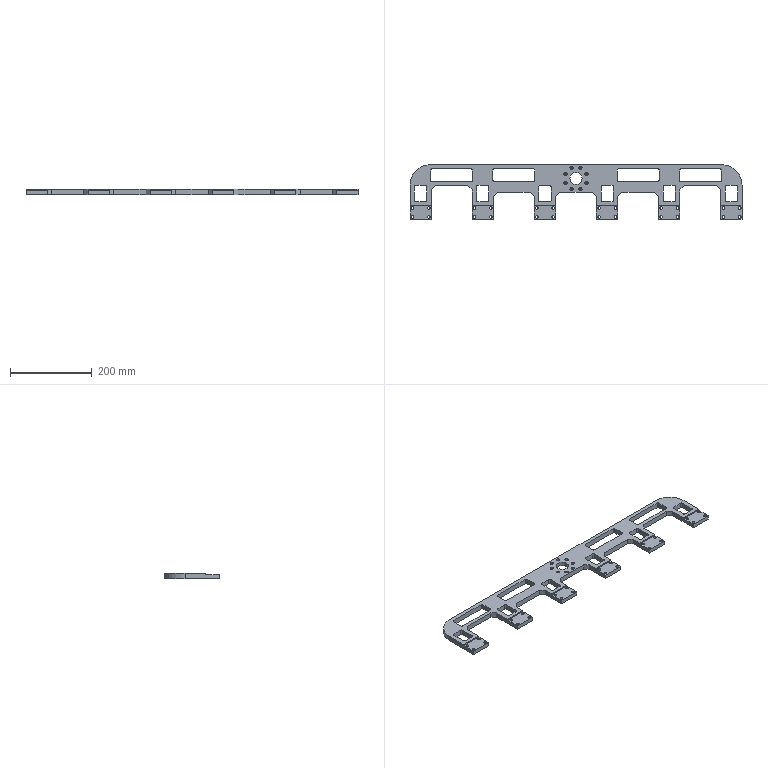Part | 1 solid | 181 faces | box 813.6 x 134 x 13 mm | volume 618398 mm3 | plane 97 | cylinder 84 | commonest cylinder face diameters 6 x40 6.5 x24 4.5 x8 8 x8 100 x2 30 x1